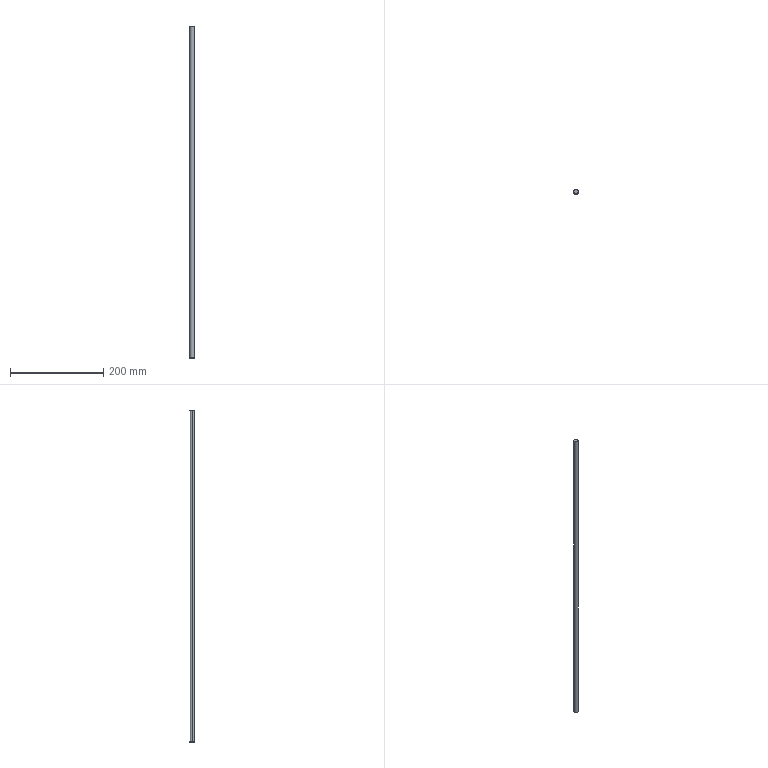Part | STEP file | PRODUCT259.stp | 1 solid | 8 faces | box 10 x 10 x 711 mm | volume 55834 mm3 | cone 4 | plane 2 | cylinder 2 | commonest cylinder face diameters 10 x2
STEP:
#1=CARTESIAN_POINT('',(0.,0.,0.));
#2=DIRECTION('',(0.,0.,1.));
#3=DIRECTION('',(1.,0.,0.));
#4=AXIS2_PLACEMENT_3D('',#1,#2,#3);
#5=CARTESIAN_POINT('',(-5.,0.,810.5));
#6=VERTEX_POINT('',#5);
#7=CARTESIAN_POINT('',(-4.5,0.,811.));
#8=VERTEX_POINT('',#7);
#9=CARTESIAN_POINT('',(-5.,0.,810.5));
#10=DIRECTION('',(0.7071,0.,0.7071));
#11=VECTOR('',#10,1.);
#12=LINE('',#9,#11);
#13=CARTESIAN_POINT('',(0.,0.,811.025));
#14=DIRECTION('',(0.,0.,-1.));
#15=DIRECTION('',(-1.,0.,0.));
#16=AXIS2_PLACEMENT_3D('',#13,#14,#15);
#17=CONICAL_SURFACE('',#16,4.475,0.7854);
#18=CARTESIAN_POINT('',(0.,0.525));
#19=DIRECTION('',(0.,-1.));
#20=VECTOR('',#19,1.);
#21=LINE('',#18,#20);
#22=(GEOMETRIC_REPRESENTATION_CONTEXT(2)PARAMETRIC_REPRESENTATION_CONTEXT()REPRESENTATION_CONTEXT('',''));
#23=DEFINITIONAL_REPRESENTATION('',(#21),#22);
#24=PCURVE('',#17,#23);
#25=CARTESIAN_POINT('',(0.,0.,811.025));
#26=DIRECTION('',(0.,0.,-1.));
#27=DIRECTION('',(-1.,0.,0.));
#28=AXIS2_PLACEMENT_3D('',#25,#26,#27);
#29=CONICAL_SURFACE('',#28,4.475,0.7854);
#30=CARTESIAN_POINT('',(6.283,0.525));
#31=DIRECTION('',(0.,-1.));
#32=VECTOR('',#31,1.);
#33=LINE('',#30,#32);
#34=(GEOMETRIC_REPRESENTATION_CONTEXT(2)PARAMETRIC_REPRESENTATION_CONTEXT()REPRESENTATION_CONTEXT('',''));
#35=DEFINITIONAL_REPRESENTATION('',(#33),#34);
#36=PCURVE('',#29,#35);
#37=SURFACE_CURVE('',#12,(#24,#36),.PCURVE_S1.);
#38=EDGE_CURVE('',#6,#8,#37,.T.);
#39=ORIENTED_EDGE('',*,*,#38,.T.);
#40=CARTESIAN_POINT('',(4.5,0.,811.));
#41=VERTEX_POINT('',#40);
#42=CARTESIAN_POINT('',(0.,0.,811.));
#43=DIRECTION('',(0.,0.,1.));
#44=DIRECTION('',(1.,0.,0.));
#45=AXIS2_PLACEMENT_3D('',#42,#43,#44);
#46=CIRCLE('',#45,4.5);
#47=CARTESIAN_POINT('',(3.142,0.025));
#48=DIRECTION('',(-1.,0.));
#49=VECTOR('',#48,1.);
#50=LINE('',#47,#49);
#51=(GEOMETRIC_REPRESENTATION_CONTEXT(2)PARAMETRIC_REPRESENTATION_CONTEXT()REPRESENTATION_CONTEXT('',''));
#52=DEFINITIONAL_REPRESENTATION('',(#50),#51);
#53=PCURVE('',#17,#52);
#54=CARTESIAN_POINT('',(-4.95,-4.95,811.));
#55=DIRECTION('',(0.,0.,1.));
#56=DIRECTION('',(1.,0.,0.));
#57=AXIS2_PLACEMENT_3D('',#54,#55,#56);
#58=PLANE('',#57);
#59=CARTESIAN_POINT('',(4.95,4.95));
#60=DIRECTION('',(1.,0.));
#61=AXIS2_PLACEMENT_2D('',#59,#60);
#62=CIRCLE('',#61,4.5);
#63=(GEOMETRIC_REPRESENTATION_CONTEXT(2)PARAMETRIC_REPRESENTATION_CONTEXT()REPRESENTATION_CONTEXT('',''));
#64=DEFINITIONAL_REPRESENTATION('',(#62),#63);
#65=PCURVE('',#58,#64);
#66=SURFACE_CURVE('',#46,(#53,#65),.PCURVE_S1.);
#67=EDGE_CURVE('',#41,#8,#66,.T.);
#68=ORIENTED_EDGE('',*,*,#67,.F.);
#69=CARTESIAN_POINT('',(5.,0.,810.5));
#70=VERTEX_POINT('',#69);
#71=CARTESIAN_POINT('',(5.,0.,810.5));
#72=DIRECTION('',(-0.7071,0.,0.7071));
#73=VECTOR('',#72,1.);
#74=LINE('',#71,#73);
#75=CARTESIAN_POINT('',(3.142,0.525));
#76=DIRECTION('',(0.,-1.));
#77=VECTOR('',#76,1.);
#78=LINE('',#75,#77);
#79=(GEOMETRIC_REPRESENTATION_CONTEXT(2)PARAMETRIC_REPRESENTATION_CONTEXT()REPRESENTATION_CONTEXT('',''));
#80=DEFINITIONAL_REPRESENTATION('',(#78),#79);
#81=PCURVE('',#17,#80);
#82=CARTESIAN_POINT('',(3.142,0.525));
#83=DIRECTION('',(0.,-1.));
#84=VECTOR('',#83,1.);
#85=LINE('',#82,#84);
#86=(GEOMETRIC_REPRESENTATION_CONTEXT(2)PARAMETRIC_REPRESENTATION_CONTEXT()REPRESENTATION_CONTEXT('',''));
#87=DEFINITIONAL_REPRESENTATION('',(#85),#86);
#88=PCURVE('',#29,#87);
#89=SURFACE_CURVE('',#74,(#81,#88),.PCURVE_S1.);
#90=EDGE_CURVE('',#70,#41,#89,.T.);
#91=ORIENTED_EDGE('',*,*,#90,.F.);
#92=CARTESIAN_POINT('',(0.,0.,810.5));
#93=DIRECTION('',(0.,0.,-1.));
#94=DIRECTION('',(1.,0.,0.));
#95=AXIS2_PLACEMENT_3D('',#92,#93,#94);
#96=CIRCLE('',#95,5.);
#97=CARTESIAN_POINT('',(-3.142,0.525));
#98=DIRECTION('',(1.,0.));
#99=VECTOR('',#98,1.);
#100=LINE('',#97,#99);
#101=(GEOMETRIC_REPRESENTATION_CONTEXT(2)PARAMETRIC_REPRESENTATION_CONTEXT()REPRESENTATION_CONTEXT('',''));
#102=DEFINITIONAL_REPRESENTATION('',(#100),#101);
#103=PCURVE('',#17,#102);
#104=CARTESIAN_POINT('',(0.,0.,511.));
#105=DIRECTION('',(0.,0.,-1.));
#106=DIRECTION('',(-1.,0.,0.));
#107=AXIS2_PLACEMENT_3D('',#104,#105,#106);
#108=CYLINDRICAL_SURFACE('',#107,5.);
#109=CARTESIAN_POINT('',(-3.142,-299.5));
#110=DIRECTION('',(1.,0.));
#111=VECTOR('',#110,1.);
#112=LINE('',#109,#111);
#113=(GEOMETRIC_REPRESENTATION_CONTEXT(2)PARAMETRIC_REPRESENTATION_CONTEXT()REPRESENTATION_CONTEXT('',''));
#114=DEFINITIONAL_REPRESENTATION('',(#112),#113);
#115=PCURVE('',#108,#114);
#116=SURFACE_CURVE('',#96,(#103,#115),.PCURVE_S1.);
#117=EDGE_CURVE('',#6,#70,#116,.T.);
#118=ORIENTED_EDGE('',*,*,#117,.F.);
#119=EDGE_LOOP('',(#39,#68,#91,#118));
#120=FACE_BOUND('',#119,.T.);
#121=ADVANCED_FACE('',(#120),#17,.T.);
#122=ORIENTED_EDGE('',*,*,#67,.T.);
#123=CARTESIAN_POINT('',(0.,0.,811.));
#124=DIRECTION('',(0.,0.,1.));
#125=DIRECTION('',(1.,0.,0.));
#126=AXIS2_PLACEMENT_3D('',#123,#124,#125);
#127=CIRCLE('',#126,4.5);
#128=CARTESIAN_POINT('',(4.95,4.95));
#129=DIRECTION('',(1.,0.));
#130=AXIS2_PLACEMENT_2D('',#128,#129);
#131=CIRCLE('',#130,4.5);
#132=(GEOMETRIC_REPRESENTATION_CONTEXT(2)PARAMETRIC_REPRESENTATION_CONTEXT()REPRESENTATION_CONTEXT('',''));
#133=DEFINITIONAL_REPRESENTATION('',(#131),#132);
#134=PCURVE('',#58,#133);
#135=CARTESIAN_POINT('',(9.425,0.025));
#136=DIRECTION('',(-1.,0.));
#137=VECTOR('',#136,1.);
#138=LINE('',#135,#137);
#139=(GEOMETRIC_REPRESENTATION_CONTEXT(2)PARAMETRIC_REPRESENTATION_CONTEXT()REPRESENTATION_CONTEXT('',''));
#140=DEFINITIONAL_REPRESENTATION('',(#138),#139);
#141=PCURVE('',#29,#140);
#142=SURFACE_CURVE('',#127,(#134,#141),.PCURVE_S1.);
#143=EDGE_CURVE('',#8,#41,#142,.T.);
#144=ORIENTED_EDGE('',*,*,#143,.T.);
#145=EDGE_LOOP('',(#122,#144));
#146=FACE_BOUND('',#145,.T.);
#147=ADVANCED_FACE('',(#146),#58,.T.);
#148=CARTESIAN_POINT('',(5.,0.,100.5));
#149=VERTEX_POINT('',#148);
#150=CARTESIAN_POINT('',(4.5,0.,100.));
#151=VERTEX_POINT('',#150);
#152=CARTESIAN_POINT('',(5.,0.,100.5));
#153=DIRECTION('',(-0.7071,0.,-0.7071));
#154=VECTOR('',#153,1.);
#155=LINE('',#152,#154);
#156=CARTESIAN_POINT('',(0.,0.,99.975));
#157=DIRECTION('',(0.,0.,1.));
#158=DIRECTION('',(1.,0.,0.));
#159=AXIS2_PLACEMENT_3D('',#156,#157,#158);
#160=CONICAL_SURFACE('',#159,4.475,0.7854);
#161=CARTESIAN_POINT('',(0.,0.525));
#162=DIRECTION('',(0.,-1.));
#163=VECTOR('',#162,1.);
#164=LINE('',#161,#163);
#165=(GEOMETRIC_REPRESENTATION_CONTEXT(2)PARAMETRIC_REPRESENTATION_CONTEXT()REPRESENTATION_CONTEXT('',''));
#166=DEFINITIONAL_REPRESENTATION('',(#164),#165);
#167=PCURVE('',#160,#166);
#168=CARTESIAN_POINT('',(0.,0.,99.975));
#169=DIRECTION('',(0.,0.,1.));
#170=DIRECTION('',(1.,0.,0.));
#171=AXIS2_PLACEMENT_3D('',#168,#169,#170);
#172=CONICAL_SURFACE('',#171,4.475,0.7854);
#173=CARTESIAN_POINT('',(6.283,0.525));
#174=DIRECTION('',(0.,-1.));
#175=VECTOR('',#174,1.);
#176=LINE('',#173,#175);
#177=(GEOMETRIC_REPRESENTATION_CONTEXT(2)PARAMETRIC_REPRESENTATION_CONTEXT()REPRESENTATION_CONTEXT('',''));
#178=DEFINITIONAL_REPRESENTATION('',(#176),#177);
#179=PCURVE('',#172,#178);
#180=SURFACE_CURVE('',#155,(#167,#179),.PCURVE_S1.);
#181=EDGE_CURVE('',#149,#151,#180,.T.);
#182=ORIENTED_EDGE('',*,*,#181,.T.);
#183=CARTESIAN_POINT('',(-4.5,0.,100.));
#184=VERTEX_POINT('',#183);
#185=CARTESIAN_POINT('',(0.,0.,100.));
#186=DIRECTION('',(0.,0.,-1.));
#187=DIRECTION('',(1.,0.,0.));
#188=AXIS2_PLACEMENT_3D('',#185,#186,#187);
#189=CIRCLE('',#188,4.5);
#190=CARTESIAN_POINT('',(6.283,0.025));
#191=DIRECTION('',(-1.,0.));
#192=VECTOR('',#191,1.);
#193=LINE('',#190,#192);
#194=(GEOMETRIC_REPRESENTATION_CONTEXT(2)PARAMETRIC_REPRESENTATION_CONTEXT()REPRESENTATION_CONTEXT('',''));
#195=DEFINITIONAL_REPRESENTATION('',(#193),#194);
#196=PCURVE('',#160,#195);
#197=CARTESIAN_POINT('',(-4.95,-4.95,100.));
#198=DIRECTION('',(0.,0.,1.));
#199=DIRECTION('',(1.,0.,0.));
#200=AXIS2_PLACEMENT_3D('',#197,#198,#199);
#201=PLANE('',#200);
#202=CARTESIAN_POINT('',(9.45,4.95));
#203=CARTESIAN_POINT('',(9.45,-2.844));
#204=CARTESIAN_POINT('',(2.7,1.053));
#205=CARTESIAN_POINT('',(-4.05,4.95));
#206=CARTESIAN_POINT('',(2.7,8.847));
#207=CARTESIAN_POINT('',(9.45,12.744));
#208=CARTESIAN_POINT('',(9.45,4.95));
#209=(BOUNDED_CURVE()B_SPLINE_CURVE(2,(#202,#203,#204,#205,#206,#207,#208),.UNSPECIFIED.,.T.,.F.)B_SPLINE_CURVE_WITH_KNOTS((1,2,2,2,2,1),(-2.094,0.,2.094,4.189,6.283,8.378),.UNSPECIFIED.)CURVE()GEOMETRIC_REPRESENTATION_ITEM()RATIONAL_B_SPLINE_CURVE((1.,0.5,1.,0.5,1.,0.5,1.))REPRESENTATION_ITEM(''));
#210=(GEOMETRIC_REPRESENTATION_CONTEXT(2)PARAMETRIC_REPRESENTATION_CONTEXT()REPRESENTATION_CONTEXT('',''));
#211=DEFINITIONAL_REPRESENTATION('',(#209),#210);
#212=PCURVE('',#201,#211);
#213=SURFACE_CURVE('',#189,(#196,#212),.PCURVE_S1.);
#214=EDGE_CURVE('',#184,#151,#213,.T.);
#215=ORIENTED_EDGE('',*,*,#214,.F.);
#216=CARTESIAN_POINT('',(-5.,0.,100.5));
#217=VERTEX_POINT('',#216);
#218=CARTESIAN_POINT('',(-5.,0.,100.5));
#219=DIRECTION('',(0.7071,0.,-0.7071));
#220=VECTOR('',#219,1.);
#221=LINE('',#218,#220);
#222=CARTESIAN_POINT('',(3.142,0.525));
#223=DIRECTION('',(0.,-1.));
#224=VECTOR('',#223,1.);
#225=LINE('',#222,#224);
#226=(GEOMETRIC_REPRESENTATION_CONTEXT(2)PARAMETRIC_REPRESENTATION_CONTEXT()REPRESENTATION_CONTEXT('',''));
#227=DEFINITIONAL_REPRESENTATION('',(#225),#226);
#228=PCURVE('',#160,#227);
#229=CARTESIAN_POINT('',(3.142,0.525));
#230=DIRECTION('',(0.,-1.));
#231=VECTOR('',#230,1.);
#232=LINE('',#229,#231);
#233=(GEOMETRIC_REPRESENTATION_CONTEXT(2)PARAMETRIC_REPRESENTATION_CONTEXT()REPRESENTATION_CONTEXT('',''));
#234=DEFINITIONAL_REPRESENTATION('',(#232),#233);
#235=PCURVE('',#172,#234);
#236=SURFACE_CURVE('',#221,(#228,#235),.PCURVE_S1.);
#237=EDGE_CURVE('',#217,#184,#236,.T.);
#238=ORIENTED_EDGE('',*,*,#237,.F.);
#239=CARTESIAN_POINT('',(0.,0.,100.5));
#240=DIRECTION('',(0.,0.,1.));
#241=DIRECTION('',(1.,0.,0.));
#242=AXIS2_PLACEMENT_3D('',#239,#240,#241);
#243=CIRCLE('',#242,5.);
#244=CARTESIAN_POINT('',(0.,0.525));
#245=DIRECTION('',(1.,0.));
#246=VECTOR('',#245,1.);
#247=LINE('',#244,#246);
#248=(GEOMETRIC_REPRESENTATION_CONTEXT(2)PARAMETRIC_REPRESENTATION_CONTEXT()REPRESENTATION_CONTEXT('',''));
#249=DEFINITIONAL_REPRESENTATION('',(#247),#248);
#250=PCURVE('',#160,#249);
#251=CARTESIAN_POINT('',(3.142,410.5));
#252=DIRECTION('',(-1.,0.));
#253=VECTOR('',#252,1.);
#254=LINE('',#251,#253);
#255=(GEOMETRIC_REPRESENTATION_CONTEXT(2)PARAMETRIC_REPRESENTATION_CONTEXT()REPRESENTATION_CONTEXT('',''));
#256=DEFINITIONAL_REPRESENTATION('',(#254),#255);
#257=PCURVE('',#108,#256);
#258=SURFACE_CURVE('',#243,(#250,#257),.PCURVE_S1.);
#259=EDGE_CURVE('',#149,#217,#258,.T.);
#260=ORIENTED_EDGE('',*,*,#259,.F.);
#261=EDGE_LOOP('',(#182,#215,#238,#260));
#262=FACE_BOUND('',#261,.T.);
#263=ADVANCED_FACE('',(#262),#160,.T.);
#264=CARTESIAN_POINT('',(0.,0.,100.));
#265=DIRECTION('',(0.,0.,-1.));
#266=DIRECTION('',(1.,0.,0.));
#267=AXIS2_PLACEMENT_3D('',#264,#265,#266);
#268=CIRCLE('',#267,4.5);
#269=CARTESIAN_POINT('',(9.45,4.95));
#270=CARTESIAN_POINT('',(9.45,-2.844));
#271=CARTESIAN_POINT('',(2.7,1.053));
#272=CARTESIAN_POINT('',(-4.05,4.95));
#273=CARTESIAN_POINT('',(2.7,8.847));
#274=CARTESIAN_POINT('',(9.45,12.744));
#275=CARTESIAN_POINT('',(9.45,4.95));
#276=(BOUNDED_CURVE()B_SPLINE_CURVE(2,(#269,#270,#271,#272,#273,#274,#275),.UNSPECIFIED.,.T.,.F.)B_SPLINE_CURVE_WITH_KNOTS((1,2,2,2,2,1),(-2.094,0.,2.094,4.189,6.283,8.378),.UNSPECIFIED.)CURVE()GEOMETRIC_REPRESENTATION_ITEM()RATIONAL_B_SPLINE_CURVE((1.,0.5,1.,0.5,1.,0.5,1.))REPRESENTATION_ITEM(''));
#277=(GEOMETRIC_REPRESENTATION_CONTEXT(2)PARAMETRIC_REPRESENTATION_CONTEXT()REPRESENTATION_CONTEXT('',''));
#278=DEFINITIONAL_REPRESENTATION('',(#276),#277);
#279=PCURVE('',#201,#278);
#280=CARTESIAN_POINT('',(6.283,0.025));
#281=DIRECTION('',(-1.,0.));
#282=VECTOR('',#281,1.);
#283=LINE('',#280,#282);
#284=(GEOMETRIC_REPRESENTATION_CONTEXT(2)PARAMETRIC_REPRESENTATION_CONTEXT()REPRESENTATION_CONTEXT('',''));
#285=DEFINITIONAL_REPRESENTATION('',(#283),#284);
#286=PCURVE('',#172,#285);
#287=SURFACE_CURVE('',#268,(#279,#286),.PCURVE_S1.);
#288=EDGE_CURVE('',#151,#184,#287,.T.);
#289=ORIENTED_EDGE('',*,*,#288,.T.);
#290=ORIENTED_EDGE('',*,*,#214,.T.);
#291=EDGE_LOOP('',(#289,#290));
#292=FACE_BOUND('',#291,.T.);
#293=ADVANCED_FACE('',(#292),#201,.F.);
#294=CARTESIAN_POINT('',(-5.,0.,100.5));
#295=DIRECTION('',(0.,0.,1.));
#296=VECTOR('',#295,1.);
#297=LINE('',#294,#296);
#298=CARTESIAN_POINT('',(0.,410.5));
#299=DIRECTION('',(0.,-1.));
#300=VECTOR('',#299,1.);
#301=LINE('',#298,#300);
#302=(GEOMETRIC_REPRESENTATION_CONTEXT(2)PARAMETRIC_REPRESENTATION_CONTEXT()REPRESENTATION_CONTEXT('',''));
#303=DEFINITIONAL_REPRESENTATION('',(#301),#302);
#304=PCURVE('',#108,#303);
#305=CARTESIAN_POINT('',(0.,0.,511.));
#306=DIRECTION('',(0.,0.,-1.));
#307=DIRECTION('',(-1.,0.,0.));
#308=AXIS2_PLACEMENT_3D('',#305,#306,#307);
#309=CYLINDRICAL_SURFACE('',#308,5.);
#310=CARTESIAN_POINT('',(6.283,410.5));
#311=DIRECTION('',(0.,-1.));
#312=VECTOR('',#311,1.);
#313=LINE('',#310,#312);
#314=(GEOMETRIC_REPRESENTATION_CONTEXT(2)PARAMETRIC_REPRESENTATION_CONTEXT()REPRESENTATION_CONTEXT('',''));
#315=DEFINITIONAL_REPRESENTATION('',(#313),#314);
#316=PCURVE('',#309,#315);
#317=SURFACE_CURVE('',#297,(#304,#316),.PCURVE_S1.);
#318=EDGE_CURVE('',#217,#6,#317,.T.);
#319=ORIENTED_EDGE('',*,*,#318,.T.);
#320=ORIENTED_EDGE('',*,*,#117,.T.);
#321=CARTESIAN_POINT('',(5.,0.,100.5));
#322=DIRECTION('',(0.,0.,1.));
#323=VECTOR('',#322,1.);
#324=LINE('',#321,#323);
#325=CARTESIAN_POINT('',(3.142,410.5));
#326=DIRECTION('',(0.,-1.));
#327=VECTOR('',#326,1.);
#328=LINE('',#325,#327);
#329=(GEOMETRIC_REPRESENTATION_CONTEXT(2)PARAMETRIC_REPRESENTATION_CONTEXT()REPRESENTATION_CONTEXT('',''));
#330=DEFINITIONAL_REPRESENTATION('',(#328),#329);
#331=PCURVE('',#108,#330);
#332=CARTESIAN_POINT('',(3.142,410.5));
#333=DIRECTION('',(0.,-1.));
#334=VECTOR('',#333,1.);
#335=LINE('',#332,#334);
#336=(GEOMETRIC_REPRESENTATION_CONTEXT(2)PARAMETRIC_REPRESENTATION_CONTEXT()REPRESENTATION_CONTEXT('',''));
#337=DEFINITIONAL_REPRESENTATION('',(#335),#336);
#338=PCURVE('',#309,#337);
#339=SURFACE_CURVE('',#324,(#331,#338),.PCURVE_S1.);
#340=EDGE_CURVE('',#149,#70,#339,.T.);
#341=ORIENTED_EDGE('',*,*,#340,.F.);
#342=ORIENTED_EDGE('',*,*,#259,.T.);
#343=EDGE_LOOP('',(#319,#320,#341,#342));
#344=FACE_BOUND('',#343,.T.);
#345=ADVANCED_FACE('',(#344),#108,.T.);
#346=ORIENTED_EDGE('',*,*,#318,.F.);
#347=CARTESIAN_POINT('',(0.,0.,100.5));
#348=DIRECTION('',(0.,0.,1.));
#349=DIRECTION('',(1.,0.,0.));
#350=AXIS2_PLACEMENT_3D('',#347,#348,#349);
#351=CIRCLE('',#350,5.);
#352=CARTESIAN_POINT('',(9.425,410.5));
#353=DIRECTION('',(-1.,0.));
#354=VECTOR('',#353,1.);
#355=LINE('',#352,#354);
#356=(GEOMETRIC_REPRESENTATION_CONTEXT(2)PARAMETRIC_REPRESENTATION_CONTEXT()REPRESENTATION_CONTEXT('',''));
#357=DEFINITIONAL_REPRESENTATION('',(#355),#356);
#358=PCURVE('',#309,#357);
#359=CARTESIAN_POINT('',(0.,0.525));
#360=DIRECTION('',(1.,0.));
#361=VECTOR('',#360,1.);
#362=LINE('',#359,#361);
#363=(GEOMETRIC_REPRESENTATION_CONTEXT(2)PARAMETRIC_REPRESENTATION_CONTEXT()REPRESENTATION_CONTEXT('',''));
#364=DEFINITIONAL_REPRESENTATION('',(#362),#363);
#365=PCURVE('',#172,#364);
#366=SURFACE_CURVE('',#351,(#358,#365),.PCURVE_S1.);
#367=EDGE_CURVE('',#217,#149,#366,.T.);
#368=ORIENTED_EDGE('',*,*,#367,.T.);
#369=ORIENTED_EDGE('',*,*,#340,.T.);
#370=CARTESIAN_POINT('',(0.,0.,810.5));
#371=DIRECTION('',(0.,0.,-1.));
#372=DIRECTION('',(1.,0.,0.));
#373=AXIS2_PLACEMENT_3D('',#370,#371,#372);
#374=CIRCLE('',#373,5.);
#375=CARTESIAN_POINT('',(3.142,-299.5));
#376=DIRECTION('',(1.,0.));
#377=VECTOR('',#376,1.);
#378=LINE('',#375,#377);
#379=(GEOMETRIC_REPRESENTATION_CONTEXT(2)PARAMETRIC_REPRESENTATION_CONTEXT()REPRESENTATION_CONTEXT('',''));
#380=DEFINITIONAL_REPRESENTATION('',(#378),#379);
#381=PCURVE('',#309,#380);
#382=CARTESIAN_POINT('',(3.142,0.525));
#383=DIRECTION('',(1.,0.));
#384=VECTOR('',#383,1.);
#385=LINE('',#382,#384);
#386=(GEOMETRIC_REPRESENTATION_CONTEXT(2)PARAMETRIC_REPRESENTATION_CONTEXT()REPRESENTATION_CONTEXT('',''));
#387=DEFINITIONAL_REPRESENTATION('',(#385),#386);
#388=PCURVE('',#29,#387);
#389=SURFACE_CURVE('',#374,(#381,#388),.PCURVE_S1.);
#390=EDGE_CURVE('',#70,#6,#389,.T.);
#391=ORIENTED_EDGE('',*,*,#390,.T.);
#392=EDGE_LOOP('',(#346,#368,#369,#391));
#393=FACE_BOUND('',#392,.T.);
#394=ADVANCED_FACE('',(#393),#309,.T.);
#395=ORIENTED_EDGE('',*,*,#181,.F.);
#396=ORIENTED_EDGE('',*,*,#367,.F.);
#397=ORIENTED_EDGE('',*,*,#237,.T.);
#398=ORIENTED_EDGE('',*,*,#288,.F.);
#399=EDGE_LOOP('',(#395,#396,#397,#398));
#400=FACE_BOUND('',#399,.T.);
#401=ADVANCED_FACE('',(#400),#172,.T.);
#402=ORIENTED_EDGE('',*,*,#38,.F.);
#403=ORIENTED_EDGE('',*,*,#390,.F.);
#404=ORIENTED_EDGE('',*,*,#90,.T.);
#405=ORIENTED_EDGE('',*,*,#143,.F.);
#406=EDGE_LOOP('',(#402,#403,#404,#405));
#407=FACE_BOUND('',#406,.T.);
#408=ADVANCED_FACE('',(#407),#29,.T.);
#409=CLOSED_SHELL('',(#121,#147,#263,#293,#345,#394,#401,#408));
#410=MANIFOLD_SOLID_BREP('',#409);
#411=(LENGTH_UNIT()NAMED_UNIT(*)SI_UNIT(.MILLI.,.METRE.));
#412=UNCERTAINTY_MEASURE_WITH_UNIT(LENGTH_MEASURE(0.0000001),#411,'','');
#413=(NAMED_UNIT(*)PLANE_ANGLE_UNIT()SI_UNIT($,.RADIAN.));
#414=(NAMED_UNIT(*)SI_UNIT($,.STERADIAN.)SOLID_ANGLE_UNIT());
#415=(GEOMETRIC_REPRESENTATION_CONTEXT(3)GLOBAL_UNCERTAINTY_ASSIGNED_CONTEXT((#412))GLOBAL_UNIT_ASSIGNED_CONTEXT((#411,#413,#414))REPRESENTATION_CONTEXT('',''));
#416=ADVANCED_BREP_SHAPE_REPRESENTATION('',(#4,#410),#415);